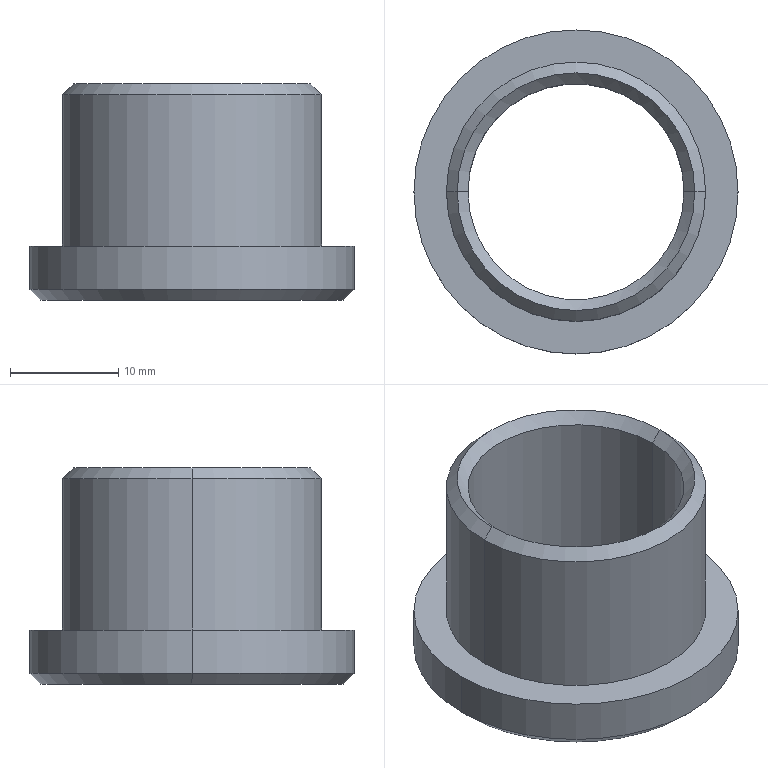Part | SolidWorks | features Chamfer 1, Extrusion 1, ICE 1 | 1 solid | 14 faces | box 30 x 30 x 20 mm | volume 3922 mm3 | cone 6 | cylinder 6 | plane 2 | commonest cylinder face diameters 20 x2 24 x2 30 x2
STEP:
#1=CARTESIAN_POINT('',(-14.,0.,0.));
#2=VERTEX_POINT('',#1);
#3=CARTESIAN_POINT('',(14.,0.,0.));
#4=VERTEX_POINT('',#3);
#5=CARTESIAN_POINT('',(0.,0.,0.));
#6=DIRECTION('',(0.,0.,-1.));
#7=DIRECTION('',(1.,0.,0.));
#8=AXIS2_PLACEMENT_3D('',#5,#6,#7);
#9=CIRCLE('',#8,14.);
#10=EDGE_CURVE('',#2,#4,#9,.T.);
#11=ORIENTED_EDGE('',*,*,#10,.F.);
#12=CARTESIAN_POINT('',(-15.,0.,1.));
#13=VERTEX_POINT('',#12);
#14=CARTESIAN_POINT('',(-15.,0.,1.));
#15=DIRECTION('',(-0.7071,0.,0.7071));
#16=VECTOR('',#15,1000.);
#17=LINE('',#14,#16);
#18=EDGE_CURVE('',#2,#13,#17,.T.);
#19=ORIENTED_EDGE('',*,*,#18,.T.);
#20=CARTESIAN_POINT('',(15.,0.,1.));
#21=VERTEX_POINT('',#20);
#22=CARTESIAN_POINT('',(0.,0.,1.));
#23=DIRECTION('',(0.,0.,1.));
#24=DIRECTION('',(1.,0.,0.));
#25=AXIS2_PLACEMENT_3D('',#22,#23,#24);
#26=CIRCLE('',#25,15.);
#27=EDGE_CURVE('',#21,#13,#26,.T.);
#28=ORIENTED_EDGE('',*,*,#27,.F.);
#29=CARTESIAN_POINT('',(15.,0.,1.));
#30=DIRECTION('',(0.7071,0.,0.7071));
#31=VECTOR('',#30,1000.);
#32=LINE('',#29,#31);
#33=EDGE_CURVE('',#4,#21,#32,.T.);
#34=ORIENTED_EDGE('',*,*,#33,.F.);
#35=EDGE_LOOP('',(#11,#19,#28,#34));
#36=FACE_OUTER_BOUND('',#35,.T.);
#37=CARTESIAN_POINT('',(0.,0.,1.));
#38=DIRECTION('',(0.,0.,1.));
#39=DIRECTION('',(1.,0.,0.));
#40=AXIS2_PLACEMENT_3D('',#37,#38,#39);
#41=CONICAL_SURFACE('',#40,15.,0.7854);
#42=ADVANCED_FACE('',(#36),#41,.T.);
#43=CARTESIAN_POINT('',(-10.,0.,19.));
#44=VERTEX_POINT('',#43);
#45=CARTESIAN_POINT('',(10.,0.,19.));
#46=VERTEX_POINT('',#45);
#47=CARTESIAN_POINT('',(0.,0.,19.));
#48=DIRECTION('',(0.,0.,1.));
#49=DIRECTION('',(1.,0.,0.));
#50=AXIS2_PLACEMENT_3D('',#47,#48,#49);
#51=CIRCLE('',#50,10.);
#52=EDGE_CURVE('',#44,#46,#51,.T.);
#53=ORIENTED_EDGE('',*,*,#52,.F.);
#54=CARTESIAN_POINT('',(-11.,0.,20.));
#55=VERTEX_POINT('',#54);
#56=CARTESIAN_POINT('',(-10.,0.,19.));
#57=DIRECTION('',(-0.7071,0.,0.7071));
#58=VECTOR('',#57,1000.);
#59=LINE('',#56,#58);
#60=EDGE_CURVE('',#44,#55,#59,.T.);
#61=ORIENTED_EDGE('',*,*,#60,.T.);
#62=CARTESIAN_POINT('',(11.,0.,20.));
#63=VERTEX_POINT('',#62);
#64=CARTESIAN_POINT('',(0.,0.,20.));
#65=DIRECTION('',(0.,0.,1.));
#66=DIRECTION('',(1.,0.,0.));
#67=AXIS2_PLACEMENT_3D('',#64,#65,#66);
#68=CIRCLE('',#67,11.);
#69=EDGE_CURVE('',#55,#63,#68,.T.);
#70=ORIENTED_EDGE('',*,*,#69,.T.);
#71=CARTESIAN_POINT('',(10.,0.,19.));
#72=DIRECTION('',(0.7071,0.,0.7071));
#73=VECTOR('',#72,1000.);
#74=LINE('',#71,#73);
#75=EDGE_CURVE('',#46,#63,#74,.T.);
#76=ORIENTED_EDGE('',*,*,#75,.F.);
#77=EDGE_LOOP('',(#53,#61,#70,#76));
#78=FACE_OUTER_BOUND('',#77,.T.);
#79=CARTESIAN_POINT('',(0.,0.,19.));
#80=DIRECTION('',(0.,0.,1.));
#81=DIRECTION('',(1.,0.,0.));
#82=AXIS2_PLACEMENT_3D('',#79,#80,#81);
#83=CONICAL_SURFACE('',#82,10.,0.7854);
#84=ADVANCED_FACE('',(#78),#83,.F.);
#85=CARTESIAN_POINT('',(0.,0.,20.));
#86=DIRECTION('',(0.,0.,1.));
#87=DIRECTION('',(1.,0.,0.));
#88=AXIS2_PLACEMENT_3D('',#85,#86,#87);
#89=CIRCLE('',#88,11.);
#90=EDGE_CURVE('',#63,#55,#89,.T.);
#91=ORIENTED_EDGE('',*,*,#90,.F.);
#92=CARTESIAN_POINT('',(12.,0.,19.));
#93=VERTEX_POINT('',#92);
#94=CARTESIAN_POINT('',(11.,0.,20.));
#95=DIRECTION('',(0.7071,0.,-0.7071));
#96=VECTOR('',#95,1000.);
#97=LINE('',#94,#96);
#98=EDGE_CURVE('',#63,#93,#97,.T.);
#99=ORIENTED_EDGE('',*,*,#98,.T.);
#100=CARTESIAN_POINT('',(-12.,0.,19.));
#101=VERTEX_POINT('',#100);
#102=CARTESIAN_POINT('',(0.,0.,19.));
#103=DIRECTION('',(0.,0.,-1.));
#104=DIRECTION('',(1.,0.,0.));
#105=AXIS2_PLACEMENT_3D('',#102,#103,#104);
#106=CIRCLE('',#105,12.);
#107=EDGE_CURVE('',#101,#93,#106,.T.);
#108=ORIENTED_EDGE('',*,*,#107,.F.);
#109=CARTESIAN_POINT('',(-11.,0.,20.));
#110=DIRECTION('',(-0.7071,0.,-0.7071));
#111=VECTOR('',#110,1000.);
#112=LINE('',#109,#111);
#113=EDGE_CURVE('',#55,#101,#112,.T.);
#114=ORIENTED_EDGE('',*,*,#113,.F.);
#115=EDGE_LOOP('',(#91,#99,#108,#114));
#116=FACE_OUTER_BOUND('',#115,.T.);
#117=CARTESIAN_POINT('',(0.,0.,20.));
#118=DIRECTION('',(0.,0.,-1.));
#119=DIRECTION('',(-1.,0.,0.));
#120=AXIS2_PLACEMENT_3D('',#117,#118,#119);
#121=CONICAL_SURFACE('',#120,11.,0.7854);
#122=ADVANCED_FACE('',(#116),#121,.T.);
#123=ORIENTED_EDGE('',*,*,#107,.T.);
#124=CARTESIAN_POINT('',(12.,0.,5.));
#125=VERTEX_POINT('',#124);
#126=CARTESIAN_POINT('',(12.,0.,20.));
#127=DIRECTION('',(0.,0.,-1.));
#128=VECTOR('',#127,1000.);
#129=LINE('',#126,#128);
#130=EDGE_CURVE('',#93,#125,#129,.T.);
#131=ORIENTED_EDGE('',*,*,#130,.T.);
#132=CARTESIAN_POINT('',(-12.,0.,5.));
#133=VERTEX_POINT('',#132);
#134=CARTESIAN_POINT('',(0.,0.,5.));
#135=DIRECTION('',(0.,0.,1.));
#136=DIRECTION('',(1.,0.,0.));
#137=AXIS2_PLACEMENT_3D('',#134,#135,#136);
#138=CIRCLE('',#137,12.);
#139=EDGE_CURVE('',#125,#133,#138,.T.);
#140=ORIENTED_EDGE('',*,*,#139,.T.);
#141=CARTESIAN_POINT('',(-12.,0.,20.));
#142=DIRECTION('',(0.,0.,-1.));
#143=VECTOR('',#142,1000.);
#144=LINE('',#141,#143);
#145=EDGE_CURVE('',#101,#133,#144,.T.);
#146=ORIENTED_EDGE('',*,*,#145,.F.);
#147=EDGE_LOOP('',(#123,#131,#140,#146));
#148=FACE_OUTER_BOUND('',#147,.T.);
#149=CARTESIAN_POINT('',(0.,0.,20.));
#150=DIRECTION('',(0.,0.,-1.));
#151=DIRECTION('',(-1.,0.,0.));
#152=AXIS2_PLACEMENT_3D('',#149,#150,#151);
#153=CYLINDRICAL_SURFACE('',#152,12.);
#154=ADVANCED_FACE('',(#148),#153,.T.);
#155=ORIENTED_EDGE('',*,*,#52,.T.);
#156=CARTESIAN_POINT('',(10.,0.,0.));
#157=VERTEX_POINT('',#156);
#158=CARTESIAN_POINT('',(10.,0.,5.));
#159=DIRECTION('',(0.,0.,-1.));
#160=VECTOR('',#159,1000.);
#161=LINE('',#158,#160);
#162=EDGE_CURVE('',#46,#157,#161,.T.);
#163=ORIENTED_EDGE('',*,*,#162,.T.);
#164=CARTESIAN_POINT('',(-10.,0.,0.));
#165=VERTEX_POINT('',#164);
#166=CARTESIAN_POINT('',(0.,0.,0.));
#167=DIRECTION('',(0.,0.,1.));
#168=DIRECTION('',(1.,0.,0.));
#169=AXIS2_PLACEMENT_3D('',#166,#167,#168);
#170=CIRCLE('',#169,10.);
#171=EDGE_CURVE('',#165,#157,#170,.T.);
#172=ORIENTED_EDGE('',*,*,#171,.F.);
#173=CARTESIAN_POINT('',(-10.,0.,5.));
#174=DIRECTION('',(0.,0.,-1.));
#175=VECTOR('',#174,1000.);
#176=LINE('',#173,#175);
#177=EDGE_CURVE('',#44,#165,#176,.T.);
#178=ORIENTED_EDGE('',*,*,#177,.F.);
#179=EDGE_LOOP('',(#155,#163,#172,#178));
#180=FACE_OUTER_BOUND('',#179,.T.);
#181=CARTESIAN_POINT('',(0.,0.,5.));
#182=DIRECTION('',(0.,0.,-1.));
#183=DIRECTION('',(-1.,0.,0.));
#184=AXIS2_PLACEMENT_3D('',#181,#182,#183);
#185=CYLINDRICAL_SURFACE('',#184,10.);
#186=ADVANCED_FACE('',(#180),#185,.F.);
#187=CARTESIAN_POINT('',(15.,0.,5.));
#188=VERTEX_POINT('',#187);
#189=CARTESIAN_POINT('',(-15.,0.,5.));
#190=VERTEX_POINT('',#189);
#191=CARTESIAN_POINT('',(0.,0.,5.));
#192=DIRECTION('',(0.,0.,1.));
#193=DIRECTION('',(1.,0.,0.));
#194=AXIS2_PLACEMENT_3D('',#191,#192,#193);
#195=CIRCLE('',#194,15.);
#196=EDGE_CURVE('',#188,#190,#195,.T.);
#197=ORIENTED_EDGE('',*,*,#196,.F.);
#198=CARTESIAN_POINT('',(15.,0.,5.));
#199=DIRECTION('',(0.,0.,-1.));
#200=VECTOR('',#199,1000.);
#201=LINE('',#198,#200);
#202=EDGE_CURVE('',#188,#21,#201,.T.);
#203=ORIENTED_EDGE('',*,*,#202,.T.);
#204=ORIENTED_EDGE('',*,*,#27,.T.);
#205=CARTESIAN_POINT('',(-15.,0.,5.));
#206=DIRECTION('',(0.,0.,-1.));
#207=VECTOR('',#206,1000.);
#208=LINE('',#205,#207);
#209=EDGE_CURVE('',#190,#13,#208,.T.);
#210=ORIENTED_EDGE('',*,*,#209,.F.);
#211=EDGE_LOOP('',(#197,#203,#204,#210));
#212=FACE_OUTER_BOUND('',#211,.T.);
#213=CARTESIAN_POINT('',(0.,0.,5.));
#214=DIRECTION('',(0.,0.,-1.));
#215=DIRECTION('',(-1.,0.,0.));
#216=AXIS2_PLACEMENT_3D('',#213,#214,#215);
#217=CYLINDRICAL_SURFACE('',#216,15.);
#218=ADVANCED_FACE('',(#212),#217,.T.);
#219=CARTESIAN_POINT('',(0.,0.,5.));
#220=DIRECTION('',(0.,0.,1.));
#221=DIRECTION('',(1.,0.,0.));
#222=AXIS2_PLACEMENT_3D('',#219,#220,#221);
#223=CIRCLE('',#222,15.);
#224=EDGE_CURVE('',#190,#188,#223,.T.);
#225=ORIENTED_EDGE('',*,*,#224,.T.);
#226=ORIENTED_EDGE('',*,*,#196,.T.);
#227=EDGE_LOOP('',(#225,#226));
#228=FACE_OUTER_BOUND('',#227,.T.);
#229=CARTESIAN_POINT('',(0.,0.,5.));
#230=DIRECTION('',(0.,0.,1.));
#231=DIRECTION('',(1.,0.,0.));
#232=AXIS2_PLACEMENT_3D('',#229,#230,#231);
#233=CIRCLE('',#232,12.);
#234=EDGE_CURVE('',#133,#125,#233,.T.);
#235=ORIENTED_EDGE('',*,*,#234,.F.);
#236=ORIENTED_EDGE('',*,*,#139,.F.);
#237=EDGE_LOOP('',(#235,#236));
#238=FACE_BOUND('',#237,.T.);
#239=CARTESIAN_POINT('',(0.,0.,5.));
#240=DIRECTION('',(0.,0.,1.));
#241=DIRECTION('',(1.,0.,0.));
#242=AXIS2_PLACEMENT_3D('',#239,#240,#241);
#243=PLANE('',#242);
#244=ADVANCED_FACE('',(#228,#238),#243,.T.);
#245=CARTESIAN_POINT('',(0.,0.,0.));
#246=DIRECTION('',(0.,0.,-1.));
#247=DIRECTION('',(1.,0.,0.));
#248=AXIS2_PLACEMENT_3D('',#245,#246,#247);
#249=CIRCLE('',#248,14.);
#250=EDGE_CURVE('',#4,#2,#249,.T.);
#251=ORIENTED_EDGE('',*,*,#250,.T.);
#252=ORIENTED_EDGE('',*,*,#10,.T.);
#253=EDGE_LOOP('',(#251,#252));
#254=FACE_OUTER_BOUND('',#253,.T.);
#255=ORIENTED_EDGE('',*,*,#171,.T.);
#256=CARTESIAN_POINT('',(0.,0.,0.));
#257=DIRECTION('',(0.,0.,1.));
#258=DIRECTION('',(1.,0.,0.));
#259=AXIS2_PLACEMENT_3D('',#256,#257,#258);
#260=CIRCLE('',#259,10.);
#261=EDGE_CURVE('',#157,#165,#260,.T.);
#262=ORIENTED_EDGE('',*,*,#261,.T.);
#263=EDGE_LOOP('',(#255,#262));
#264=FACE_BOUND('',#263,.T.);
#265=CARTESIAN_POINT('',(0.,0.,0.));
#266=DIRECTION('',(0.,0.,1.));
#267=DIRECTION('',(1.,0.,0.));
#268=AXIS2_PLACEMENT_3D('',#265,#266,#267);
#269=PLANE('',#268);
#270=ADVANCED_FACE('',(#254,#264),#269,.F.);
#271=ORIENTED_EDGE('',*,*,#202,.F.);
#272=ORIENTED_EDGE('',*,*,#224,.F.);
#273=ORIENTED_EDGE('',*,*,#209,.T.);
#274=CARTESIAN_POINT('',(0.,0.,1.));
#275=DIRECTION('',(0.,0.,1.));
#276=DIRECTION('',(1.,0.,0.));
#277=AXIS2_PLACEMENT_3D('',#274,#275,#276);
#278=CIRCLE('',#277,15.);
#279=EDGE_CURVE('',#13,#21,#278,.T.);
#280=ORIENTED_EDGE('',*,*,#279,.T.);
#281=EDGE_LOOP('',(#271,#272,#273,#280));
#282=FACE_OUTER_BOUND('',#281,.T.);
#283=CARTESIAN_POINT('',(0.,0.,5.));
#284=DIRECTION('',(0.,0.,-1.));
#285=DIRECTION('',(-1.,0.,0.));
#286=AXIS2_PLACEMENT_3D('',#283,#284,#285);
#287=CYLINDRICAL_SURFACE('',#286,15.);
#288=ADVANCED_FACE('',(#282),#287,.T.);
#289=ORIENTED_EDGE('',*,*,#162,.F.);
#290=CARTESIAN_POINT('',(0.,0.,19.));
#291=DIRECTION('',(0.,0.,1.));
#292=DIRECTION('',(1.,0.,0.));
#293=AXIS2_PLACEMENT_3D('',#290,#291,#292);
#294=CIRCLE('',#293,10.);
#295=EDGE_CURVE('',#46,#44,#294,.T.);
#296=ORIENTED_EDGE('',*,*,#295,.T.);
#297=ORIENTED_EDGE('',*,*,#177,.T.);
#298=ORIENTED_EDGE('',*,*,#261,.F.);
#299=EDGE_LOOP('',(#289,#296,#297,#298));
#300=FACE_OUTER_BOUND('',#299,.T.);
#301=CARTESIAN_POINT('',(0.,0.,5.));
#302=DIRECTION('',(0.,0.,-1.));
#303=DIRECTION('',(-1.,0.,0.));
#304=AXIS2_PLACEMENT_3D('',#301,#302,#303);
#305=CYLINDRICAL_SURFACE('',#304,10.);
#306=ADVANCED_FACE('',(#300),#305,.F.);
#307=ORIENTED_EDGE('',*,*,#130,.F.);
#308=CARTESIAN_POINT('',(0.,0.,19.));
#309=DIRECTION('',(0.,0.,-1.));
#310=DIRECTION('',(1.,0.,0.));
#311=AXIS2_PLACEMENT_3D('',#308,#309,#310);
#312=CIRCLE('',#311,12.);
#313=EDGE_CURVE('',#93,#101,#312,.T.);
#314=ORIENTED_EDGE('',*,*,#313,.T.);
#315=ORIENTED_EDGE('',*,*,#145,.T.);
#316=ORIENTED_EDGE('',*,*,#234,.T.);
#317=EDGE_LOOP('',(#307,#314,#315,#316));
#318=FACE_OUTER_BOUND('',#317,.T.);
#319=CARTESIAN_POINT('',(0.,0.,20.));
#320=DIRECTION('',(0.,0.,-1.));
#321=DIRECTION('',(-1.,0.,0.));
#322=AXIS2_PLACEMENT_3D('',#319,#320,#321);
#323=CYLINDRICAL_SURFACE('',#322,12.);
#324=ADVANCED_FACE('',(#318),#323,.T.);
#325=ORIENTED_EDGE('',*,*,#98,.F.);
#326=ORIENTED_EDGE('',*,*,#69,.F.);
#327=ORIENTED_EDGE('',*,*,#113,.T.);
#328=ORIENTED_EDGE('',*,*,#313,.F.);
#329=EDGE_LOOP('',(#325,#326,#327,#328));
#330=FACE_OUTER_BOUND('',#329,.T.);
#331=CARTESIAN_POINT('',(0.,0.,20.));
#332=DIRECTION('',(0.,0.,-1.));
#333=DIRECTION('',(-1.,0.,0.));
#334=AXIS2_PLACEMENT_3D('',#331,#332,#333);
#335=CONICAL_SURFACE('',#334,11.,0.7854);
#336=ADVANCED_FACE('',(#330),#335,.T.);
#337=ORIENTED_EDGE('',*,*,#60,.F.);
#338=ORIENTED_EDGE('',*,*,#295,.F.);
#339=ORIENTED_EDGE('',*,*,#75,.T.);
#340=ORIENTED_EDGE('',*,*,#90,.T.);
#341=EDGE_LOOP('',(#337,#338,#339,#340));
#342=FACE_OUTER_BOUND('',#341,.T.);
#343=CARTESIAN_POINT('',(0.,0.,19.));
#344=DIRECTION('',(0.,0.,1.));
#345=DIRECTION('',(1.,0.,0.));
#346=AXIS2_PLACEMENT_3D('',#343,#344,#345);
#347=CONICAL_SURFACE('',#346,10.,0.7854);
#348=ADVANCED_FACE('',(#342),#347,.F.);
#349=ORIENTED_EDGE('',*,*,#18,.F.);
#350=ORIENTED_EDGE('',*,*,#250,.F.);
#351=ORIENTED_EDGE('',*,*,#33,.T.);
#352=ORIENTED_EDGE('',*,*,#279,.F.);
#353=EDGE_LOOP('',(#349,#350,#351,#352));
#354=FACE_OUTER_BOUND('',#353,.T.);
#355=CARTESIAN_POINT('',(0.,0.,1.));
#356=DIRECTION('',(0.,0.,1.));
#357=DIRECTION('',(1.,0.,0.));
#358=AXIS2_PLACEMENT_3D('',#355,#356,#357);
#359=CONICAL_SURFACE('',#358,15.,0.7854);
#360=ADVANCED_FACE('',(#354),#359,.T.);
#361=CLOSED_SHELL('',(#42,#84,#122,#154,#186,#218,#244,#270,#288,#306,#324,#336,#348,#360));
#362=MANIFOLD_SOLID_BREP('',#361);
#363=CARTESIAN_POINT('',(0.,0.,0.));
#364=DIRECTION('',(0.,0.,1.));
#365=DIRECTION('',(1.,0.,0.));
#366=AXIS2_PLACEMENT_3D('',#363,#364,#365);
#367=(LENGTH_UNIT()NAMED_UNIT(*)SI_UNIT(.MILLI.,.METRE.));
#368=UNCERTAINTY_MEASURE_WITH_UNIT(LENGTH_MEASURE(0.00001),#367,'','');
#369=(NAMED_UNIT(*)PLANE_ANGLE_UNIT()SI_UNIT($,.RADIAN.));
#370=(NAMED_UNIT(*)SI_UNIT($,.STERADIAN.)SOLID_ANGLE_UNIT());
#371=(GEOMETRIC_REPRESENTATION_CONTEXT(3)GLOBAL_UNCERTAINTY_ASSIGNED_CONTEXT((#368))GLOBAL_UNIT_ASSIGNED_CONTEXT((#367,#369,#370))REPRESENTATION_CONTEXT('',''));
#372=ADVANCED_BREP_SHAPE_REPRESENTATION('',(#362,#366),#371);